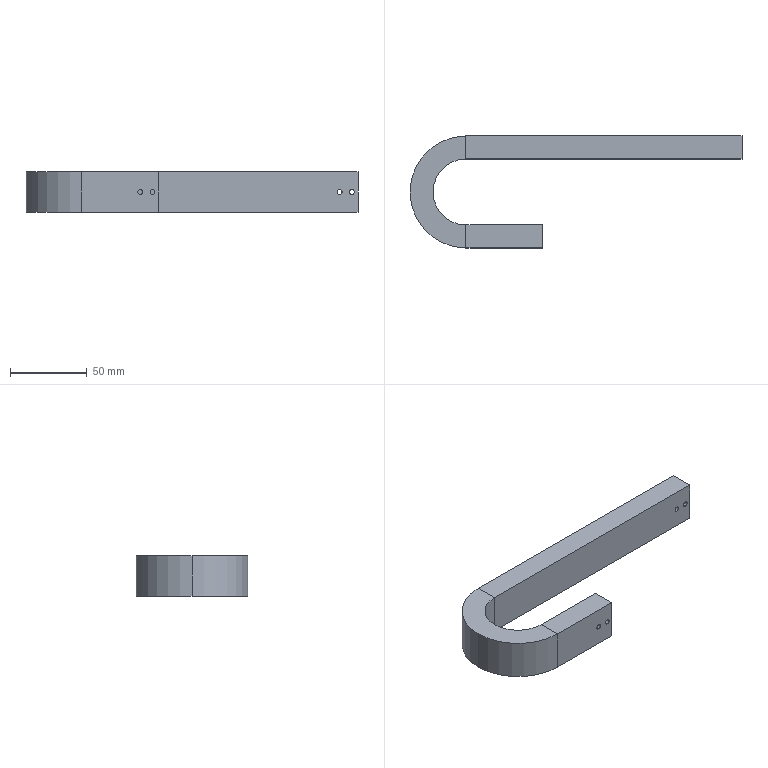Part | NX | features BREP 1 | 1 solid | 50 faces | box 216.5 x 73 x 26.5 mm | volume 63258 mm3 | cylinder 24 | plane 22 | cone 4 | commonest cylinder face diameters 3.2 x16 43 x2 48 x2 68 x2 73 x2
STEP:
#1=CARTESIAN_POINT('',(126.,53.,1.6));
#2=VERTEX_POINT('',#1);
#3=CARTESIAN_POINT('',(126.,50.5,1.6));
#4=VERTEX_POINT('',#3);
#5=CARTESIAN_POINT('',(126.,50.5,1.6));
#6=DIRECTION('',(0.,-1.,0.));
#7=VECTOR('',#6,1000.);
#8=LINE('',#5,#7);
#9=EDGE_CURVE('',#2,#4,#8,.T.);
#10=ORIENTED_EDGE('',*,*,#9,.F.);
#11=CARTESIAN_POINT('',(126.,53.,-1.6));
#12=VERTEX_POINT('',#11);
#13=CARTESIAN_POINT('',(126.,53.,0.));
#14=DIRECTION('',(0.,-1.,0.));
#15=DIRECTION('',(0.,0.,-1.));
#16=AXIS2_PLACEMENT_3D('',#13,#14,#15);
#17=CIRCLE('',#16,1.6);
#18=EDGE_CURVE('',#12,#2,#17,.T.);
#19=ORIENTED_EDGE('',*,*,#18,.F.);
#20=CARTESIAN_POINT('',(126.,50.5,-1.6));
#21=VERTEX_POINT('',#20);
#22=CARTESIAN_POINT('',(126.,50.5,-1.6));
#23=DIRECTION('',(0.,-1.,0.));
#24=VECTOR('',#23,1000.);
#25=LINE('',#22,#24);
#26=EDGE_CURVE('',#12,#21,#25,.T.);
#27=ORIENTED_EDGE('',*,*,#26,.T.);
#28=CARTESIAN_POINT('',(126.,50.5,0.));
#29=DIRECTION('',(0.,-1.,0.));
#30=DIRECTION('',(0.,0.,-1.));
#31=AXIS2_PLACEMENT_3D('',#28,#29,#30);
#32=CIRCLE('',#31,1.6);
#33=EDGE_CURVE('',#21,#4,#32,.T.);
#34=ORIENTED_EDGE('',*,*,#33,.T.);
#35=EDGE_LOOP('',(#10,#19,#27,#34));
#36=FACE_BOUND('',#35,.T.);
#37=CARTESIAN_POINT('',(126.,50.5,0.));
#38=DIRECTION('',(0.,-1.,0.));
#39=DIRECTION('',(0.,0.,-1.));
#40=AXIS2_PLACEMENT_3D('',#37,#38,#39);
#41=CYLINDRICAL_SURFACE('',#40,1.6);
#42=ADVANCED_FACE('',(#36),#41,.F.);
#43=CARTESIAN_POINT('',(126.,65.499,1.6));
#44=VERTEX_POINT('',#43);
#45=CARTESIAN_POINT('',(126.,63.,1.6));
#46=VERTEX_POINT('',#45);
#47=CARTESIAN_POINT('',(126.,50.5,1.6));
#48=DIRECTION('',(0.,-1.,0.));
#49=VECTOR('',#48,1000.);
#50=LINE('',#47,#49);
#51=EDGE_CURVE('',#44,#46,#50,.T.);
#52=ORIENTED_EDGE('',*,*,#51,.F.);
#53=CARTESIAN_POINT('',(126.,65.499,-1.6));
#54=VERTEX_POINT('',#53);
#55=CARTESIAN_POINT('',(126.,65.499,0.));
#56=DIRECTION('',(0.,-1.,0.));
#57=DIRECTION('',(0.,0.,-1.));
#58=AXIS2_PLACEMENT_3D('',#55,#56,#57);
#59=CIRCLE('',#58,1.6);
#60=EDGE_CURVE('',#54,#44,#59,.T.);
#61=ORIENTED_EDGE('',*,*,#60,.F.);
#62=CARTESIAN_POINT('',(126.,63.,-1.6));
#63=VERTEX_POINT('',#62);
#64=CARTESIAN_POINT('',(126.,50.5,-1.6));
#65=DIRECTION('',(0.,-1.,0.));
#66=VECTOR('',#65,1000.);
#67=LINE('',#64,#66);
#68=EDGE_CURVE('',#54,#63,#67,.T.);
#69=ORIENTED_EDGE('',*,*,#68,.T.);
#70=CARTESIAN_POINT('',(126.,63.,0.));
#71=DIRECTION('',(0.,1.,0.));
#72=DIRECTION('',(0.,0.,1.));
#73=AXIS2_PLACEMENT_3D('',#70,#71,#72);
#74=CIRCLE('',#73,1.6);
#75=EDGE_CURVE('',#46,#63,#74,.T.);
#76=ORIENTED_EDGE('',*,*,#75,.F.);
#77=EDGE_LOOP('',(#52,#61,#69,#76));
#78=FACE_BOUND('',#77,.T.);
#79=CARTESIAN_POINT('',(126.,50.5,0.));
#80=DIRECTION('',(0.,-1.,0.));
#81=DIRECTION('',(0.,0.,-1.));
#82=AXIS2_PLACEMENT_3D('',#79,#80,#81);
#83=CYLINDRICAL_SURFACE('',#82,1.6);
#84=ADVANCED_FACE('',(#78),#83,.F.);
#85=CARTESIAN_POINT('',(126.,65.5,1.598));
#86=VERTEX_POINT('',#85);
#87=CARTESIAN_POINT('',(126.,65.499,1.6));
#88=DIRECTION('',(0.,-0.515,0.8572));
#89=VECTOR('',#88,1000.);
#90=LINE('',#87,#89);
#91=EDGE_CURVE('',#86,#44,#90,.T.);
#92=ORIENTED_EDGE('',*,*,#91,.F.);
#93=CARTESIAN_POINT('',(126.,65.5,-1.598));
#94=VERTEX_POINT('',#93);
#95=CARTESIAN_POINT('',(126.,65.5,0.));
#96=DIRECTION('',(0.,-1.,0.));
#97=DIRECTION('',(0.,0.,-1.));
#98=AXIS2_PLACEMENT_3D('',#95,#96,#97);
#99=CIRCLE('',#98,1.598);
#100=EDGE_CURVE('',#94,#86,#99,.T.);
#101=ORIENTED_EDGE('',*,*,#100,.F.);
#102=CARTESIAN_POINT('',(126.,65.499,-1.6));
#103=DIRECTION('',(0.,-0.515,-0.8572));
#104=VECTOR('',#103,1000.);
#105=LINE('',#102,#104);
#106=EDGE_CURVE('',#94,#54,#105,.T.);
#107=ORIENTED_EDGE('',*,*,#106,.T.);
#108=ORIENTED_EDGE('',*,*,#60,.T.);
#109=EDGE_LOOP('',(#92,#101,#107,#108));
#110=FACE_BOUND('',#109,.T.);
#111=CARTESIAN_POINT('',(126.,65.499,0.));
#112=DIRECTION('',(0.,-1.,0.));
#113=DIRECTION('',(0.,0.,-1.));
#114=AXIS2_PLACEMENT_3D('',#111,#112,#113);
#115=CONICAL_SURFACE('',#114,1.6,1.03);
#116=ADVANCED_FACE('',(#110),#115,.F.);
#117=CARTESIAN_POINT('',(118.,65.499,1.6));
#118=VERTEX_POINT('',#117);
#119=CARTESIAN_POINT('',(118.,63.,1.6));
#120=VERTEX_POINT('',#119);
#121=CARTESIAN_POINT('',(118.,50.5,1.6));
#122=DIRECTION('',(0.,-1.,0.));
#123=VECTOR('',#122,1000.);
#124=LINE('',#121,#123);
#125=EDGE_CURVE('',#118,#120,#124,.T.);
#126=ORIENTED_EDGE('',*,*,#125,.F.);
#127=CARTESIAN_POINT('',(118.,65.499,-1.6));
#128=VERTEX_POINT('',#127);
#129=CARTESIAN_POINT('',(118.,65.499,0.));
#130=DIRECTION('',(0.,-1.,0.));
#131=DIRECTION('',(0.,0.,-1.));
#132=AXIS2_PLACEMENT_3D('',#129,#130,#131);
#133=CIRCLE('',#132,1.6);
#134=EDGE_CURVE('',#128,#118,#133,.T.);
#135=ORIENTED_EDGE('',*,*,#134,.F.);
#136=CARTESIAN_POINT('',(118.,63.,-1.6));
#137=VERTEX_POINT('',#136);
#138=CARTESIAN_POINT('',(118.,50.5,-1.6));
#139=DIRECTION('',(0.,-1.,0.));
#140=VECTOR('',#139,1000.);
#141=LINE('',#138,#140);
#142=EDGE_CURVE('',#128,#137,#141,.T.);
#143=ORIENTED_EDGE('',*,*,#142,.T.);
#144=CARTESIAN_POINT('',(118.,63.,0.));
#145=DIRECTION('',(0.,1.,0.));
#146=DIRECTION('',(0.,0.,1.));
#147=AXIS2_PLACEMENT_3D('',#144,#145,#146);
#148=CIRCLE('',#147,1.6);
#149=EDGE_CURVE('',#120,#137,#148,.T.);
#150=ORIENTED_EDGE('',*,*,#149,.F.);
#151=EDGE_LOOP('',(#126,#135,#143,#150));
#152=FACE_BOUND('',#151,.T.);
#153=CARTESIAN_POINT('',(118.,50.5,0.));
#154=DIRECTION('',(0.,-1.,0.));
#155=DIRECTION('',(0.,0.,-1.));
#156=AXIS2_PLACEMENT_3D('',#153,#154,#155);
#157=CYLINDRICAL_SURFACE('',#156,1.6);
#158=ADVANCED_FACE('',(#152),#157,.F.);
#159=CARTESIAN_POINT('',(118.,65.5,1.598));
#160=VERTEX_POINT('',#159);
#161=CARTESIAN_POINT('',(118.,65.499,1.6));
#162=DIRECTION('',(0.,-0.515,0.8572));
#163=VECTOR('',#162,1000.);
#164=LINE('',#161,#163);
#165=EDGE_CURVE('',#160,#118,#164,.T.);
#166=ORIENTED_EDGE('',*,*,#165,.F.);
#167=CARTESIAN_POINT('',(118.,65.5,-1.598));
#168=VERTEX_POINT('',#167);
#169=CARTESIAN_POINT('',(118.,65.5,0.));
#170=DIRECTION('',(0.,-1.,0.));
#171=DIRECTION('',(0.,0.,-1.));
#172=AXIS2_PLACEMENT_3D('',#169,#170,#171);
#173=CIRCLE('',#172,1.598);
#174=EDGE_CURVE('',#168,#160,#173,.T.);
#175=ORIENTED_EDGE('',*,*,#174,.F.);
#176=CARTESIAN_POINT('',(118.,65.499,-1.6));
#177=DIRECTION('',(0.,-0.515,-0.8572));
#178=VECTOR('',#177,1000.);
#179=LINE('',#176,#178);
#180=EDGE_CURVE('',#168,#128,#179,.T.);
#181=ORIENTED_EDGE('',*,*,#180,.T.);
#182=ORIENTED_EDGE('',*,*,#134,.T.);
#183=EDGE_LOOP('',(#166,#175,#181,#182));
#184=FACE_BOUND('',#183,.T.);
#185=CARTESIAN_POINT('',(118.,65.499,0.));
#186=DIRECTION('',(0.,-1.,0.));
#187=DIRECTION('',(0.,0.,-1.));
#188=AXIS2_PLACEMENT_3D('',#185,#186,#187);
#189=CONICAL_SURFACE('',#188,1.6,1.03);
#190=ADVANCED_FACE('',(#184),#189,.F.);
#191=CARTESIAN_POINT('',(118.,53.,1.6));
#192=VERTEX_POINT('',#191);
#193=CARTESIAN_POINT('',(118.,50.5,1.6));
#194=VERTEX_POINT('',#193);
#195=CARTESIAN_POINT('',(118.,50.5,1.6));
#196=DIRECTION('',(0.,-1.,0.));
#197=VECTOR('',#196,1000.);
#198=LINE('',#195,#197);
#199=EDGE_CURVE('',#192,#194,#198,.T.);
#200=ORIENTED_EDGE('',*,*,#199,.F.);
#201=CARTESIAN_POINT('',(118.,53.,-1.6));
#202=VERTEX_POINT('',#201);
#203=CARTESIAN_POINT('',(118.,53.,0.));
#204=DIRECTION('',(0.,-1.,0.));
#205=DIRECTION('',(0.,0.,-1.));
#206=AXIS2_PLACEMENT_3D('',#203,#204,#205);
#207=CIRCLE('',#206,1.6);
#208=EDGE_CURVE('',#202,#192,#207,.T.);
#209=ORIENTED_EDGE('',*,*,#208,.F.);
#210=CARTESIAN_POINT('',(118.,50.5,-1.6));
#211=VERTEX_POINT('',#210);
#212=CARTESIAN_POINT('',(118.,50.5,-1.6));
#213=DIRECTION('',(0.,-1.,0.));
#214=VECTOR('',#213,1000.);
#215=LINE('',#212,#214);
#216=EDGE_CURVE('',#202,#211,#215,.T.);
#217=ORIENTED_EDGE('',*,*,#216,.T.);
#218=CARTESIAN_POINT('',(118.,50.5,0.));
#219=DIRECTION('',(0.,-1.,0.));
#220=DIRECTION('',(0.,0.,-1.));
#221=AXIS2_PLACEMENT_3D('',#218,#219,#220);
#222=CIRCLE('',#221,1.6);
#223=EDGE_CURVE('',#211,#194,#222,.T.);
#224=ORIENTED_EDGE('',*,*,#223,.T.);
#225=EDGE_LOOP('',(#200,#209,#217,#224));
#226=FACE_BOUND('',#225,.T.);
#227=CARTESIAN_POINT('',(118.,50.5,0.));
#228=DIRECTION('',(0.,-1.,0.));
#229=DIRECTION('',(0.,0.,-1.));
#230=AXIS2_PLACEMENT_3D('',#227,#228,#229);
#231=CYLINDRICAL_SURFACE('',#230,1.6);
#232=ADVANCED_FACE('',(#226),#231,.F.);
#233=CARTESIAN_POINT('',(-4.,7.5,1.6));
#234=VERTEX_POINT('',#233);
#235=CARTESIAN_POINT('',(-4.,5.,1.6));
#236=VERTEX_POINT('',#235);
#237=CARTESIAN_POINT('',(-4.,-7.5,1.6));
#238=DIRECTION('',(0.,-1.,0.));
#239=VECTOR('',#238,1000.);
#240=LINE('',#237,#239);
#241=EDGE_CURVE('',#234,#236,#240,.T.);
#242=ORIENTED_EDGE('',*,*,#241,.F.);
#243=CARTESIAN_POINT('',(-4.,7.5,-1.6));
#244=VERTEX_POINT('',#243);
#245=CARTESIAN_POINT('',(-4.,7.5,0.));
#246=DIRECTION('',(0.,1.,0.));
#247=DIRECTION('',(1.,0.,0.));
#248=AXIS2_PLACEMENT_3D('',#245,#246,#247);
#249=CIRCLE('',#248,1.6);
#250=EDGE_CURVE('',#234,#244,#249,.T.);
#251=ORIENTED_EDGE('',*,*,#250,.T.);
#252=CARTESIAN_POINT('',(-4.,5.,-1.6));
#253=VERTEX_POINT('',#252);
#254=CARTESIAN_POINT('',(-4.,-7.5,-1.6));
#255=DIRECTION('',(0.,-1.,0.));
#256=VECTOR('',#255,1000.);
#257=LINE('',#254,#256);
#258=EDGE_CURVE('',#244,#253,#257,.T.);
#259=ORIENTED_EDGE('',*,*,#258,.T.);
#260=CARTESIAN_POINT('',(-4.,5.,0.));
#261=DIRECTION('',(0.,1.,0.));
#262=DIRECTION('',(-1.,0.,0.));
#263=AXIS2_PLACEMENT_3D('',#260,#261,#262);
#264=CIRCLE('',#263,1.6);
#265=EDGE_CURVE('',#236,#253,#264,.T.);
#266=ORIENTED_EDGE('',*,*,#265,.F.);
#267=EDGE_LOOP('',(#242,#251,#259,#266));
#268=FACE_BOUND('',#267,.T.);
#269=CARTESIAN_POINT('',(-4.,-7.5,0.));
#270=DIRECTION('',(0.,-1.,0.));
#271=DIRECTION('',(0.,0.,-1.));
#272=AXIS2_PLACEMENT_3D('',#269,#270,#271);
#273=CYLINDRICAL_SURFACE('',#272,1.6);
#274=ADVANCED_FACE('',(#268),#273,.F.);
#275=CARTESIAN_POINT('',(-4.,-5.,1.6));
#276=VERTEX_POINT('',#275);
#277=CARTESIAN_POINT('',(-4.,-7.5,1.6));
#278=VERTEX_POINT('',#277);
#279=CARTESIAN_POINT('',(-4.,-7.5,1.6));
#280=DIRECTION('',(0.,-1.,0.));
#281=VECTOR('',#280,1000.);
#282=LINE('',#279,#281);
#283=EDGE_CURVE('',#276,#278,#282,.T.);
#284=ORIENTED_EDGE('',*,*,#283,.F.);
#285=CARTESIAN_POINT('',(-4.,-5.,-1.6));
#286=VERTEX_POINT('',#285);
#287=CARTESIAN_POINT('',(-4.,-5.,0.));
#288=DIRECTION('',(0.,-1.,0.));
#289=DIRECTION('',(1.,0.,0.));
#290=AXIS2_PLACEMENT_3D('',#287,#288,#289);
#291=CIRCLE('',#290,1.6);
#292=EDGE_CURVE('',#286,#276,#291,.T.);
#293=ORIENTED_EDGE('',*,*,#292,.F.);
#294=CARTESIAN_POINT('',(-4.,-7.5,-1.6));
#295=VERTEX_POINT('',#294);
#296=CARTESIAN_POINT('',(-4.,-7.5,-1.6));
#297=DIRECTION('',(0.,-1.,0.));
#298=VECTOR('',#297,1000.);
#299=LINE('',#296,#298);
#300=EDGE_CURVE('',#286,#295,#299,.T.);
#301=ORIENTED_EDGE('',*,*,#300,.T.);
#302=CARTESIAN_POINT('',(-4.,-7.5,0.));
#303=DIRECTION('',(0.,-1.,0.));
#304=DIRECTION('',(0.,0.,-1.));
#305=AXIS2_PLACEMENT_3D('',#302,#303,#304);
#306=CIRCLE('',#305,1.6);
#307=EDGE_CURVE('',#295,#278,#306,.T.);
#308=ORIENTED_EDGE('',*,*,#307,.T.);
#309=EDGE_LOOP('',(#284,#293,#301,#308));
#310=FACE_BOUND('',#309,.T.);
#311=CARTESIAN_POINT('',(-4.,-7.5,0.));
#312=DIRECTION('',(0.,-1.,0.));
#313=DIRECTION('',(0.,0.,-1.));
#314=AXIS2_PLACEMENT_3D('',#311,#312,#313);
#315=CYLINDRICAL_SURFACE('',#314,1.6);
#316=ADVANCED_FACE('',(#310),#315,.F.);
#317=CARTESIAN_POINT('',(-12.,7.5,1.6));
#318=VERTEX_POINT('',#317);
#319=CARTESIAN_POINT('',(-12.,5.,1.6));
#320=VERTEX_POINT('',#319);
#321=CARTESIAN_POINT('',(-12.,-7.5,1.6));
#322=DIRECTION('',(0.,-1.,0.));
#323=VECTOR('',#322,1000.);
#324=LINE('',#321,#323);
#325=EDGE_CURVE('',#318,#320,#324,.T.);
#326=ORIENTED_EDGE('',*,*,#325,.F.);
#327=CARTESIAN_POINT('',(-12.,7.5,-1.6));
#328=VERTEX_POINT('',#327);
#329=CARTESIAN_POINT('',(-12.,7.5,0.));
#330=DIRECTION('',(0.,1.,0.));
#331=DIRECTION('',(1.,0.,0.));
#332=AXIS2_PLACEMENT_3D('',#329,#330,#331);
#333=CIRCLE('',#332,1.6);
#334=EDGE_CURVE('',#318,#328,#333,.T.);
#335=ORIENTED_EDGE('',*,*,#334,.T.);
#336=CARTESIAN_POINT('',(-12.,5.,-1.6));
#337=VERTEX_POINT('',#336);
#338=CARTESIAN_POINT('',(-12.,-7.5,-1.6));
#339=DIRECTION('',(0.,-1.,0.));
#340=VECTOR('',#339,1000.);
#341=LINE('',#338,#340);
#342=EDGE_CURVE('',#328,#337,#341,.T.);
#343=ORIENTED_EDGE('',*,*,#342,.T.);
#344=CARTESIAN_POINT('',(-12.,5.,0.));
#345=DIRECTION('',(0.,1.,0.));
#346=DIRECTION('',(-1.,0.,0.));
#347=AXIS2_PLACEMENT_3D('',#344,#345,#346);
#348=CIRCLE('',#347,1.6);
#349=EDGE_CURVE('',#320,#337,#348,.T.);
#350=ORIENTED_EDGE('',*,*,#349,.F.);
#351=EDGE_LOOP('',(#326,#335,#343,#350));
#352=FACE_BOUND('',#351,.T.);
#353=CARTESIAN_POINT('',(-12.,-7.5,0.));
#354=DIRECTION('',(0.,-1.,0.));
#355=DIRECTION('',(0.,0.,-1.));
#356=AXIS2_PLACEMENT_3D('',#353,#354,#355);
#357=CYLINDRICAL_SURFACE('',#356,1.6);
#358=ADVANCED_FACE('',(#352),#357,.F.);
#359=CARTESIAN_POINT('',(-12.,-5.,1.6));
#360=VERTEX_POINT('',#359);
#361=CARTESIAN_POINT('',(-12.,-7.5,1.6));
#362=VERTEX_POINT('',#361);
#363=CARTESIAN_POINT('',(-12.,-7.5,1.6));
#364=DIRECTION('',(0.,-1.,0.));
#365=VECTOR('',#364,1000.);
#366=LINE('',#363,#365);
#367=EDGE_CURVE('',#360,#362,#366,.T.);
#368=ORIENTED_EDGE('',*,*,#367,.F.);
#369=CARTESIAN_POINT('',(-12.,-5.,-1.6));
#370=VERTEX_POINT('',#369);
#371=CARTESIAN_POINT('',(-12.,-5.,0.));
#372=DIRECTION('',(0.,-1.,0.));
#373=DIRECTION('',(1.,0.,0.));
#374=AXIS2_PLACEMENT_3D('',#371,#372,#373);
#375=CIRCLE('',#374,1.6);
#376=EDGE_CURVE('',#370,#360,#375,.T.);
#377=ORIENTED_EDGE('',*,*,#376,.F.);
#378=CARTESIAN_POINT('',(-12.,-7.5,-1.6));
#379=VERTEX_POINT('',#378);
#380=CARTESIAN_POINT('',(-12.,-7.5,-1.6));
#381=DIRECTION('',(0.,-1.,0.));
#382=VECTOR('',#381,1000.);
#383=LINE('',#380,#382);
#384=EDGE_CURVE('',#370,#379,#383,.T.);
#385=ORIENTED_EDGE('',*,*,#384,.T.);
#386=CARTESIAN_POINT('',(-12.,-7.5,0.));
#387=DIRECTION('',(0.,-1.,0.));
#388=DIRECTION('',(0.,0.,-1.));
#389=AXIS2_PLACEMENT_3D('',#386,#387,#388);
#390=CIRCLE('',#389,1.6);
#391=EDGE_CURVE('',#379,#362,#390,.T.);
#392=ORIENTED_EDGE('',*,*,#391,.T.);
#393=EDGE_LOOP('',(#368,#377,#385,#392));
#394=FACE_BOUND('',#393,.T.);
#395=CARTESIAN_POINT('',(-12.,-7.5,0.));
#396=DIRECTION('',(0.,-1.,0.));
#397=DIRECTION('',(0.,0.,-1.));
#398=AXIS2_PLACEMENT_3D('',#395,#396,#397);
#399=CYLINDRICAL_SURFACE('',#398,1.6);
#400=ADVANCED_FACE('',(#394),#399,.F.);
#401=CARTESIAN_POINT('',(0.,7.5,-13.25));
#402=VERTEX_POINT('',#401);
#403=CARTESIAN_POINT('',(-50.,7.5,-13.25));
#404=VERTEX_POINT('',#403);
#405=CARTESIAN_POINT('',(0.,7.5,-13.25));
#406=DIRECTION('',(-1.,0.,0.));
#407=VECTOR('',#406,1000.);
#408=LINE('',#405,#407);
#409=EDGE_CURVE('',#402,#404,#408,.T.);
#410=ORIENTED_EDGE('',*,*,#409,.F.);
#411=CARTESIAN_POINT('',(0.,-7.5,-13.25));
#412=VERTEX_POINT('',#411);
#413=CARTESIAN_POINT('',(0.,-7.5,-13.25));
#414=DIRECTION('',(0.,1.,0.));
#415=VECTOR('',#414,1000.);
#416=LINE('',#413,#415);
#417=EDGE_CURVE('',#412,#402,#416,.T.);
#418=ORIENTED_EDGE('',*,*,#417,.F.);
#419=CARTESIAN_POINT('',(-50.,-7.5,-13.25));
#420=VERTEX_POINT('',#419);
#421=CARTESIAN_POINT('',(0.,-7.5,-13.25));
#422=DIRECTION('',(-1.,0.,0.));
#423=VECTOR('',#422,1000.);
#424=LINE('',#421,#423);
#425=EDGE_CURVE('',#412,#420,#424,.T.);
#426=ORIENTED_EDGE('',*,*,#425,.T.);
#427=CARTESIAN_POINT('',(-50.,-7.5,-13.25));
#428=DIRECTION('',(0.,1.,0.));
#429=VECTOR('',#428,1000.);
#430=LINE('',#427,#429);
#431=EDGE_CURVE('',#420,#404,#430,.T.);
#432=ORIENTED_EDGE('',*,*,#431,.T.);
#433=EDGE_LOOP('',(#410,#418,#426,#432));
#434=FACE_BOUND('',#433,.T.);
#435=CARTESIAN_POINT('',(0.,-7.5,-13.25));
#436=DIRECTION('',(0.,0.,1.));
#437=DIRECTION('',(1.,0.,0.));
#438=AXIS2_PLACEMENT_3D('',#435,#436,#437);
#439=PLANE('',#438);
#440=ADVANCED_FACE('',(#434),#439,.F.);
#441=CARTESIAN_POINT('',(0.,-7.5,13.25));
#442=VERTEX_POINT('',#441);
#443=CARTESIAN_POINT('',(-50.,-7.5,13.25));
#444=VERTEX_POINT('',#443);
#445=CARTESIAN_POINT('',(0.,-7.5,13.25));
#446=DIRECTION('',(-1.,0.,0.));
#447=VECTOR('',#446,1000.);
#448=LINE('',#445,#447);
#449=EDGE_CURVE('',#442,#444,#448,.T.);
#450=ORIENTED_EDGE('',*,*,#449,.F.);
#451=CARTESIAN_POINT('',(0.,7.5,13.25));
#452=VERTEX_POINT('',#451);
#453=CARTESIAN_POINT('',(0.,-7.5,13.25));
#454=DIRECTION('',(0.,-1.,0.));
#455=VECTOR('',#454,1000.);
#456=LINE('',#453,#455);
#457=EDGE_CURVE('',#452,#442,#456,.T.);
#458=ORIENTED_EDGE('',*,*,#457,.F.);
#459=CARTESIAN_POINT('',(-50.,7.5,13.25));
#460=VERTEX_POINT('',#459);
#461=CARTESIAN_POINT('',(0.,7.5,13.25));
#462=DIRECTION('',(-1.,0.,0.));
#463=VECTOR('',#462,1000.);
#464=LINE('',#461,#463);
#465=EDGE_CURVE('',#452,#460,#464,.T.);
#466=ORIENTED_EDGE('',*,*,#465,.T.);
#467=CARTESIAN_POINT('',(-50.,-7.5,13.25));
#468=DIRECTION('',(0.,-1.,0.));
#469=VECTOR('',#468,1000.);
#470=LINE('',#467,#469);
#471=EDGE_CURVE('',#460,#444,#470,.T.);
#472=ORIENTED_EDGE('',*,*,#471,.T.);
#473=EDGE_LOOP('',(#450,#458,#466,#472));
#474=FACE_BOUND('',#473,.T.);
#475=CARTESIAN_POINT('',(0.,-7.5,13.25));
#476=DIRECTION('',(0.,0.,-1.));
#477=DIRECTION('',(-1.,0.,0.));
#478=AXIS2_PLACEMENT_3D('',#475,#476,#477);
#479=PLANE('',#478);
#480=ADVANCED_FACE('',(#474),#479,.F.);
#481=CARTESIAN_POINT('',(-50.,-7.5,13.25));
#482=DIRECTION('',(0.,0.,-1.));
#483=VECTOR('',#482,1000.);
#484=LINE('',#481,#483);
#485=EDGE_CURVE('',#444,#420,#484,.T.);
#486=ORIENTED_EDGE('',*,*,#485,.T.);
#487=ORIENTED_EDGE('',*,*,#425,.F.);
#488=CARTESIAN_POINT('',(0.,-7.5,13.25));
#489=DIRECTION('',(0.,0.,-1.));
#490=VECTOR('',#489,1000.);
#491=LINE('',#488,#490);
#492=EDGE_CURVE('',#442,#412,#491,.T.);
#493=ORIENTED_EDGE('',*,*,#492,.F.);
#494=ORIENTED_EDGE('',*,*,#449,.T.);
#495=EDGE_LOOP('',(#486,#487,#493,#494));
#496=FACE_BOUND('',#495,.T.);
#497=ORIENTED_EDGE('',*,*,#391,.F.);
#498=CARTESIAN_POINT('',(-12.,-7.5,0.));
#499=DIRECTION('',(0.,-1.,0.));
#500=DIRECTION('',(0.,0.,-1.));
#501=AXIS2_PLACEMENT_3D('',#498,#499,#500);
#502=CIRCLE('',#501,1.6);
#503=EDGE_CURVE('',#362,#379,#502,.T.);
#504=ORIENTED_EDGE('',*,*,#503,.F.);
#505=EDGE_LOOP('',(#497,#504));
#506=FACE_BOUND('',#505,.T.);
#507=ORIENTED_EDGE('',*,*,#307,.F.);
#508=CARTESIAN_POINT('',(-4.,-7.5,0.));
#509=DIRECTION('',(0.,-1.,0.));
#510=DIRECTION('',(0.,0.,-1.));
#511=AXIS2_PLACEMENT_3D('',#508,#509,#510);
#512=CIRCLE('',#511,1.6);
#513=EDGE_CURVE('',#278,#295,#512,.T.);
#514=ORIENTED_EDGE('',*,*,#513,.F.);
#515=EDGE_LOOP('',(#507,#514));
#516=FACE_BOUND('',#515,.T.);
#517=CARTESIAN_POINT('',(0.,-7.5,13.25));
#518=DIRECTION('',(0.,1.,0.));
#519=DIRECTION('',(-1.,0.,0.));
#520=AXIS2_PLACEMENT_3D('',#517,#518,#519);
#521=PLANE('',#520);
#522=ADVANCED_FACE('',(#496,#506,#516),#521,.F.);
#523=CARTESIAN_POINT('',(-71.5,29.,-13.25));
#524=VERTEX_POINT('',#523);
#525=CARTESIAN_POINT('',(-50.,29.,-13.25));
#526=DIRECTION('',(0.,0.,-1.));
#527=DIRECTION('',(0.,-1.,0.));
#528=AXIS2_PLACEMENT_3D('',#525,#526,#527);
#529=CIRCLE('',#528,21.5);
#530=EDGE_CURVE('',#404,#524,#529,.T.);
#531=ORIENTED_EDGE('',*,*,#530,.F.);
#532=ORIENTED_EDGE('',*,*,#431,.F.);
#533=CARTESIAN_POINT('',(-86.5,29.,-13.25));
#534=VERTEX_POINT('',#533);
#535=CARTESIAN_POINT('',(-50.,29.,-13.25));
#536=DIRECTION('',(0.,0.,-1.));
#537=DIRECTION('',(0.,-1.,0.));
#538=AXIS2_PLACEMENT_3D('',#535,#536,#537);
#539=CIRCLE('',#538,36.5);
#540=EDGE_CURVE('',#420,#534,#539,.T.);
#541=ORIENTED_EDGE('',*,*,#540,.T.);
#542=CARTESIAN_POINT('',(-50.,65.5,-13.25));
#543=VERTEX_POINT('',#542);
#544=CARTESIAN_POINT('',(-50.,29.,-13.25));
#545=DIRECTION('',(0.,0.,-1.));
#546=DIRECTION('',(0.,-1.,0.));
#547=AXIS2_PLACEMENT_3D('',#544,#545,#546);
#548=CIRCLE('',#547,36.5);
#549=EDGE_CURVE('',#534,#543,#548,.T.);
#550=ORIENTED_EDGE('',*,*,#549,.T.);
#551=CARTESIAN_POINT('',(-50.,50.5,-13.25));
#552=VERTEX_POINT('',#551);
#553=CARTESIAN_POINT('',(-50.,65.5,-13.25));
#554=DIRECTION('',(0.,-1.,0.));
#555=VECTOR('',#554,1000.);
#556=LINE('',#553,#555);
#557=EDGE_CURVE('',#543,#552,#556,.T.);
#558=ORIENTED_EDGE('',*,*,#557,.T.);
#559=CARTESIAN_POINT('',(-50.,29.,-13.25));
#560=DIRECTION('',(0.,0.,-1.));
#561=DIRECTION('',(0.,-1.,0.));
#562=AXIS2_PLACEMENT_3D('',#559,#560,#561);
#563=CIRCLE('',#562,21.5);
#564=EDGE_CURVE('',#524,#552,#563,.T.);
#565=ORIENTED_EDGE('',*,*,#564,.F.);
#566=EDGE_LOOP('',(#531,#532,#541,#550,#558,#565));
#567=FACE_BOUND('',#566,.T.);
#568=CARTESIAN_POINT('',(-50.,-7.5,-13.25));
#569=DIRECTION('',(0.,0.,1.));
#570=DIRECTION('',(1.,0.,0.));
#571=AXIS2_PLACEMENT_3D('',#568,#569,#570);
#572=PLANE('',#571);
#573=ADVANCED_FACE('',(#567),#572,.F.);
#574=CARTESIAN_POINT('',(-71.5,29.,13.25));
#575=VERTEX_POINT('',#574);
#576=CARTESIAN_POINT('',(-71.5,29.,0.));
#577=DIRECTION('',(0.,0.,-1.));
#578=VECTOR('',#577,1000.);
#579=LINE('',#576,#578);
#580=EDGE_CURVE('',#575,#524,#579,.T.);
#581=ORIENTED_EDGE('',*,*,#580,.F.);
#582=CARTESIAN_POINT('',(-50.,29.,13.25));
#583=DIRECTION('',(0.,0.,-1.));
#584=DIRECTION('',(0.,-1.,0.));
#585=AXIS2_PLACEMENT_3D('',#582,#583,#584);
#586=CIRCLE('',#585,21.5);
#587=EDGE_CURVE('',#460,#575,#586,.T.);
#588=ORIENTED_EDGE('',*,*,#587,.F.);
#589=CARTESIAN_POINT('',(-50.,7.5,13.25));
#590=DIRECTION('',(0.,0.,1.));
#591=VECTOR('',#590,1000.);
#592=LINE('',#589,#591);
#593=EDGE_CURVE('',#404,#460,#592,.T.);
#594=ORIENTED_EDGE('',*,*,#593,.F.);
#595=ORIENTED_EDGE('',*,*,#530,.T.);
#596=EDGE_LOOP('',(#581,#588,#594,#595));
#597=FACE_BOUND('',#596,.T.);
#598=CARTESIAN_POINT('',(-50.,29.,0.));
#599=DIRECTION('',(0.,0.,-1.));
#600=DIRECTION('',(-1.,0.,0.));
#601=AXIS2_PLACEMENT_3D('',#598,#599,#600);
#602=CYLINDRICAL_SURFACE('',#601,21.5);
#603=ADVANCED_FACE('',(#597),#602,.F.);
#604=CARTESIAN_POINT('',(-86.5,29.,13.25));
#605=VERTEX_POINT('',#604);
#606=CARTESIAN_POINT('',(-50.,29.,13.25));
#607=DIRECTION('',(0.,0.,-1.));
#608=DIRECTION('',(0.,-1.,0.));
#609=AXIS2_PLACEMENT_3D('',#606,#607,#608);
#610=CIRCLE('',#609,36.5);
#611=EDGE_CURVE('',#444,#605,#610,.T.);
#612=ORIENTED_EDGE('',*,*,#611,.F.);
#613=ORIENTED_EDGE('',*,*,#471,.F.);
#614=ORIENTED_EDGE('',*,*,#587,.T.);
#615=CARTESIAN_POINT('',(-50.,50.5,13.25));
#616=VERTEX_POINT('',#615);
#617=CARTESIAN_POINT('',(-50.,29.,13.25));
#618=DIRECTION('',(0.,0.,-1.));
#619=DIRECTION('',(0.,-1.,0.));
#620=AXIS2_PLACEMENT_3D('',#617,#618,#619);
#621=CIRCLE('',#620,21.5);
#622=EDGE_CURVE('',#575,#616,#621,.T.);
#623=ORIENTED_EDGE('',*,*,#622,.T.);
#624=CARTESIAN_POINT('',(-50.,65.5,13.25));
#625=VERTEX_POINT('',#624);
#626=CARTESIAN_POINT('',(-50.,65.5,13.25));
#627=DIRECTION('',(0.,1.,0.));
#628=VECTOR('',#627,1000.);
#629=LINE('',#626,#628);
#630=EDGE_CURVE('',#616,#625,#629,.T.);
#631=ORIENTED_EDGE('',*,*,#630,.T.);
#632=CARTESIAN_POINT('',(-50.,29.,13.25));
#633=DIRECTION('',(0.,0.,-1.));
#634=DIRECTION('',(0.,-1.,0.));
#635=AXIS2_PLACEMENT_3D('',#632,#633,#634);
#636=CIRCLE('',#635,36.5);
#637=EDGE_CURVE('',#605,#625,#636,.T.);
#638=ORIENTED_EDGE('',*,*,#637,.F.);
#639=EDGE_LOOP('',(#612,#613,#614,#623,#631,#638));
#640=FACE_BOUND('',#639,.T.);
#641=CARTESIAN_POINT('',(-50.,-7.5,13.25));
#642=DIRECTION('',(0.,0.,-1.));
#643=DIRECTION('',(-1.,0.,0.));
#644=AXIS2_PLACEMENT_3D('',#641,#642,#643);
#645=PLANE('',#644);
#646=ADVANCED_FACE('',(#640),#645,.F.);
#647=CARTESIAN_POINT('',(-86.5,29.,0.));
#648=DIRECTION('',(0.,0.,-1.));
#649=VECTOR('',#648,1000.);
#650=LINE('',#647,#649);
#651=EDGE_CURVE('',#605,#534,#650,.T.);
#652=ORIENTED_EDGE('',*,*,#651,.F.);
#653=ORIENTED_EDGE('',*,*,#637,.T.);
#654=CARTESIAN_POINT('',(-50.,65.5,13.25));
#655=DIRECTION('',(0.,0.,-1.));
#656=VECTOR('',#655,1000.);
#657=LINE('',#654,#656);
#658=EDGE_CURVE('',#625,#543,#657,.T.);
#659=ORIENTED_EDGE('',*,*,#658,.T.);
#660=ORIENTED_EDGE('',*,*,#549,.F.);
#661=EDGE_LOOP('',(#652,#653,#659,#660));
#662=FACE_BOUND('',#661,.T.);
#663=CARTESIAN_POINT('',(-50.,29.,0.));
#664=DIRECTION('',(0.,0.,-1.));
#665=DIRECTION('',(-1.,0.,0.));
#666=AXIS2_PLACEMENT_3D('',#663,#664,#665);
#667=CYLINDRICAL_SURFACE('',#666,36.5);
#668=ADVANCED_FACE('',(#662),#667,.T.);
#669=CARTESIAN_POINT('',(130.,50.5,-13.25));
#670=VERTEX_POINT('',#669);
#671=CARTESIAN_POINT('',(-50.,50.5,-13.25));
#672=DIRECTION('',(1.,0.,0.));
#673=VECTOR('',#672,1000.);
#674=LINE('',#671,#673);
#675=EDGE_CURVE('',#552,#670,#674,.T.);
#676=ORIENTED_EDGE('',*,*,#675,.F.);
#677=ORIENTED_EDGE('',*,*,#557,.F.);
#678=CARTESIAN_POINT('',(130.,65.5,-13.25));
#679=VERTEX_POINT('',#678);
#680=CARTESIAN_POINT('',(-50.,65.5,-13.25));
#681=DIRECTION('',(1.,0.,0.));
#682=VECTOR('',#681,1000.);
#683=LINE('',#680,#682);
#684=EDGE_CURVE('',#543,#679,#683,.T.);
#685=ORIENTED_EDGE('',*,*,#684,.T.);
#686=CARTESIAN_POINT('',(130.,65.5,-13.25));
#687=DIRECTION('',(0.,-1.,0.));
#688=VECTOR('',#687,1000.);
#689=LINE('',#686,#688);
#690=EDGE_CURVE('',#679,#670,#689,.T.);
#691=ORIENTED_EDGE('',*,*,#690,.T.);
#692=EDGE_LOOP('',(#676,#677,#685,#691));
#693=FACE_BOUND('',#692,.T.);
#694=CARTESIAN_POINT('',(-50.,65.5,-13.25));
#695=DIRECTION('',(0.,0.,1.));
#696=DIRECTION('',(1.,0.,0.));
#697=AXIS2_PLACEMENT_3D('',#694,#695,#696);
#698=PLANE('',#697);
#699=ADVANCED_FACE('',(#693),#698,.F.);
#700=CARTESIAN_POINT('',(130.,50.5,13.25));
#701=VERTEX_POINT('',#700);
#702=CARTESIAN_POINT('',(-50.,50.5,13.25));
#703=DIRECTION('',(1.,0.,0.));
#704=VECTOR('',#703,1000.);
#705=LINE('',#702,#704);
#706=EDGE_CURVE('',#616,#701,#705,.T.);
#707=ORIENTED_EDGE('',*,*,#706,.F.);
#708=CARTESIAN_POINT('',(-50.,50.5,13.25));
#709=DIRECTION('',(0.,0.,1.));
#710=VECTOR('',#709,1000.);
#711=LINE('',#708,#710);
#712=EDGE_CURVE('',#552,#616,#711,.T.);
#713=ORIENTED_EDGE('',*,*,#712,.F.);
#714=ORIENTED_EDGE('',*,*,#675,.T.);
#715=CARTESIAN_POINT('',(130.,50.5,13.25));
#716=DIRECTION('',(0.,0.,1.));
#717=VECTOR('',#716,1000.);
#718=LINE('',#715,#717);
#719=EDGE_CURVE('',#670,#701,#718,.T.);
#720=ORIENTED_EDGE('',*,*,#719,.T.);
#721=EDGE_LOOP('',(#707,#713,#714,#720));
#722=FACE_BOUND('',#721,.T.);
#723=ORIENTED_EDGE('',*,*,#223,.F.);
#724=CARTESIAN_POINT('',(118.,50.5,0.));
#725=DIRECTION('',(0.,-1.,0.));
#726=DIRECTION('',(0.,0.,-1.));
#727=AXIS2_PLACEMENT_3D('',#724,#725,#726);
#728=CIRCLE('',#727,1.6);
#729=EDGE_CURVE('',#194,#211,#728,.T.);
#730=ORIENTED_EDGE('',*,*,#729,.F.);
#731=EDGE_LOOP('',(#723,#730));
#732=FACE_BOUND('',#731,.T.);
#733=ORIENTED_EDGE('',*,*,#33,.F.);
#734=CARTESIAN_POINT('',(126.,50.5,0.));
#735=DIRECTION('',(0.,-1.,0.));
#736=DIRECTION('',(0.,0.,-1.));
#737=AXIS2_PLACEMENT_3D('',#734,#735,#736);
#738=CIRCLE('',#737,1.6);
#739=EDGE_CURVE('',#4,#21,#738,.T.);
#740=ORIENTED_EDGE('',*,*,#739,.F.);
#741=EDGE_LOOP('',(#733,#740));
#742=FACE_BOUND('',#741,.T.);
#743=CARTESIAN_POINT('',(-50.,50.5,13.25));
#744=DIRECTION('',(0.,1.,0.));
#745=DIRECTION('',(0.,0.,1.));
#746=AXIS2_PLACEMENT_3D('',#743,#744,#745);
#747=PLANE('',#746);
#748=ADVANCED_FACE('',(#722,#732,#742),#747,.F.);
#749=CARTESIAN_POINT('',(130.,65.5,13.25));
#750=VERTEX_POINT('',#749);
#751=CARTESIAN_POINT('',(-50.,65.5,13.25));
#752=DIRECTION('',(1.,0.,0.));
#753=VECTOR('',#752,1000.);
#754=LINE('',#751,#753);
#755=EDGE_CURVE('',#625,#750,#754,.T.);
#756=ORIENTED_EDGE('',*,*,#755,.F.);
#757=ORIENTED_EDGE('',*,*,#630,.F.);
#758=ORIENTED_EDGE('',*,*,#706,.T.);
#759=CARTESIAN_POINT('',(130.,65.5,13.25));
#760=DIRECTION('',(0.,1.,0.));
#761=VECTOR('',#760,1000.);
#762=LINE('',#759,#761);
#763=EDGE_CURVE('',#701,#750,#762,.T.);
#764=ORIENTED_EDGE('',*,*,#763,.T.);
#765=EDGE_LOOP('',(#756,#757,#758,#764));
#766=FACE_BOUND('',#765,.T.);
#767=CARTESIAN_POINT('',(-50.,65.5,13.25));
#768=DIRECTION('',(0.,0.,-1.));
#769=DIRECTION('',(-1.,0.,0.));
#770=AXIS2_PLACEMENT_3D('',#767,#768,#769);
#771=PLANE('',#770);
#772=ADVANCED_FACE('',(#766),#771,.F.);
#773=CARTESIAN_POINT('',(130.,65.5,13.25));
#774=DIRECTION('',(0.,0.,-1.));
#775=VECTOR('',#774,1000.);
#776=LINE('',#773,#775);
#777=EDGE_CURVE('',#750,#679,#776,.T.);
#778=ORIENTED_EDGE('',*,*,#777,.T.);
#779=ORIENTED_EDGE('',*,*,#684,.F.);
#780=ORIENTED_EDGE('',*,*,#658,.F.);
#781=ORIENTED_EDGE('',*,*,#755,.T.);
#782=EDGE_LOOP('',(#778,#779,#780,#781));
#783=FACE_BOUND('',#782,.T.);
#784=ORIENTED_EDGE('',*,*,#174,.T.);
#785=CARTESIAN_POINT('',(118.,65.5,0.));
#786=DIRECTION('',(0.,-1.,0.));
#787=DIRECTION('',(0.,0.,-1.));
#788=AXIS2_PLACEMENT_3D('',#785,#786,#787);
#789=CIRCLE('',#788,1.598);
#790=EDGE_CURVE('',#160,#168,#789,.T.);
#791=ORIENTED_EDGE('',*,*,#790,.T.);
#792=EDGE_LOOP('',(#784,#791));
#793=FACE_BOUND('',#792,.T.);
#794=ORIENTED_EDGE('',*,*,#100,.T.);
#795=CARTESIAN_POINT('',(126.,65.5,0.));
#796=DIRECTION('',(0.,-1.,0.));
#797=DIRECTION('',(0.,0.,-1.));
#798=AXIS2_PLACEMENT_3D('',#795,#796,#797);
#799=CIRCLE('',#798,1.598);
#800=EDGE_CURVE('',#86,#94,#799,.T.);
#801=ORIENTED_EDGE('',*,*,#800,.T.);
#802=EDGE_LOOP('',(#794,#801));
#803=FACE_BOUND('',#802,.T.);
#804=CARTESIAN_POINT('',(-50.,65.5,13.25));
#805=DIRECTION('',(0.,-1.,0.));
#806=DIRECTION('',(0.,0.,-1.));
#807=AXIS2_PLACEMENT_3D('',#804,#805,#806);
#808=PLANE('',#807);
#809=ADVANCED_FACE('',(#783,#793,#803),#808,.F.);
#810=CARTESIAN_POINT('',(0.,5.,-10.));
#811=VERTEX_POINT('',#810);
#812=CARTESIAN_POINT('',(0.,-5.,-10.));
#813=VERTEX_POINT('',#812);
#814=CARTESIAN_POINT('',(0.,-5.,-10.));
#815=DIRECTION('',(0.,-1.,0.));
#816=VECTOR('',#815,1000.);
#817=LINE('',#814,#816);
#818=EDGE_CURVE('',#811,#813,#817,.T.);
#819=ORIENTED_EDGE('',*,*,#818,.T.);
#820=CARTESIAN_POINT('',(0.,-5.,10.));
#821=VERTEX_POINT('',#820);
#822=CARTESIAN_POINT('',(0.,-5.,10.));
#823=DIRECTION('',(0.,0.,1.));
#824=VECTOR('',#823,1000.);
#825=LINE('',#822,#824);
#826=EDGE_CURVE('',#813,#821,#825,.T.);
#827=ORIENTED_EDGE('',*,*,#826,.T.);
#828=CARTESIAN_POINT('',(0.,5.,10.));
#829=VERTEX_POINT('',#828);
#830=CARTESIAN_POINT('',(0.,-5.,10.));
#831=DIRECTION('',(0.,1.,0.));
#832=VECTOR('',#831,1000.);
#833=LINE('',#830,#832);
#834=EDGE_CURVE('',#821,#829,#833,.T.);
#835=ORIENTED_EDGE('',*,*,#834,.T.);
#836=CARTESIAN_POINT('',(0.,5.,10.));
#837=DIRECTION('',(0.,0.,-1.));
#838=VECTOR('',#837,1000.);
#839=LINE('',#836,#838);
#840=EDGE_CURVE('',#829,#811,#839,.T.);
#841=ORIENTED_EDGE('',*,*,#840,.T.);
#842=EDGE_LOOP('',(#819,#827,#835,#841));
#843=FACE_BOUND('',#842,.T.);
#844=ORIENTED_EDGE('',*,*,#417,.T.);
#845=CARTESIAN_POINT('',(0.,7.5,13.25));
#846=DIRECTION('',(0.,0.,1.));
#847=VECTOR('',#846,1000.);
#848=LINE('',#845,#847);
#849=EDGE_CURVE('',#402,#452,#848,.T.);
#850=ORIENTED_EDGE('',*,*,#849,.T.);
#851=ORIENTED_EDGE('',*,*,#457,.T.);
#852=ORIENTED_EDGE('',*,*,#492,.T.);
#853=EDGE_LOOP('',(#844,#850,#851,#852));
#854=FACE_BOUND('',#853,.T.);
#855=CARTESIAN_POINT('',(0.,0.,0.));
#856=DIRECTION('',(-1.,0.,0.));
#857=DIRECTION('',(0.,0.,1.));
#858=AXIS2_PLACEMENT_3D('',#855,#856,#857);
#859=PLANE('',#858);
#860=ADVANCED_FACE('',(#843,#854),#859,.F.);
#861=CARTESIAN_POINT('',(130.,53.,-10.));
#862=VERTEX_POINT('',#861);
#863=CARTESIAN_POINT('',(130.,63.,-10.));
#864=VERTEX_POINT('',#863);
#865=CARTESIAN_POINT('',(130.,63.,-10.));
#866=DIRECTION('',(0.,1.,0.));
#867=VECTOR('',#866,1000.);
#868=LINE('',#865,#867);
#869=EDGE_CURVE('',#862,#864,#868,.T.);
#870=ORIENTED_EDGE('',*,*,#869,.F.);
#871=CARTESIAN_POINT('',(130.,53.,10.));
#872=VERTEX_POINT('',#871);
#873=CARTESIAN_POINT('',(130.,53.,10.));
#874=DIRECTION('',(0.,0.,-1.));
#875=VECTOR('',#874,1000.);
#876=LINE('',#873,#875);
#877=EDGE_CURVE('',#872,#862,#876,.T.);
#878=ORIENTED_EDGE('',*,*,#877,.F.);
#879=CARTESIAN_POINT('',(130.,63.,10.));
#880=VERTEX_POINT('',#879);
#881=CARTESIAN_POINT('',(130.,63.,10.));
#882=DIRECTION('',(0.,-1.,0.));
#883=VECTOR('',#882,1000.);
#884=LINE('',#881,#883);
#885=EDGE_CURVE('',#880,#872,#884,.T.);
#886=ORIENTED_EDGE('',*,*,#885,.F.);
#887=CARTESIAN_POINT('',(130.,63.,10.));
#888=DIRECTION('',(0.,0.,1.));
#889=VECTOR('',#888,1000.);
#890=LINE('',#887,#889);
#891=EDGE_CURVE('',#864,#880,#890,.T.);
#892=ORIENTED_EDGE('',*,*,#891,.F.);
#893=EDGE_LOOP('',(#870,#878,#886,#892));
#894=FACE_BOUND('',#893,.T.);
#895=ORIENTED_EDGE('',*,*,#690,.F.);
#896=ORIENTED_EDGE('',*,*,#777,.F.);
#897=ORIENTED_EDGE('',*,*,#763,.F.);
#898=ORIENTED_EDGE('',*,*,#719,.F.);
#899=EDGE_LOOP('',(#895,#896,#897,#898));
#900=FACE_BOUND('',#899,.T.);
#901=CARTESIAN_POINT('',(130.,58.,0.));
#902=DIRECTION('',(1.,0.,0.));
#903=DIRECTION('',(0.,0.,1.));
#904=AXIS2_PLACEMENT_3D('',#901,#902,#903);
#905=PLANE('',#904);
#906=ADVANCED_FACE('',(#894,#900),#905,.T.);
#907=CARTESIAN_POINT('',(-50.,-5.,10.));
#908=VERTEX_POINT('',#907);
#909=CARTESIAN_POINT('',(0.,-5.,10.));
#910=DIRECTION('',(-1.,0.,0.));
#911=VECTOR('',#910,1000.);
#912=LINE('',#909,#911);
#913=EDGE_CURVE('',#821,#908,#912,.T.);
#914=ORIENTED_EDGE('',*,*,#913,.F.);
#915=ORIENTED_EDGE('',*,*,#826,.F.);
#916=CARTESIAN_POINT('',(-50.,-5.,-10.));
#917=VERTEX_POINT('',#916);
#918=CARTESIAN_POINT('',(0.,-5.,-10.));
#919=DIRECTION('',(-1.,0.,0.));
#920=VECTOR('',#919,1000.);
#921=LINE('',#918,#920);
#922=EDGE_CURVE('',#813,#917,#921,.T.);
#923=ORIENTED_EDGE('',*,*,#922,.T.);
#924=CARTESIAN_POINT('',(-50.,-5.,10.));
#925=DIRECTION('',(0.,0.,1.));
#926=VECTOR('',#925,1000.);
#927=LINE('',#924,#926);
#928=EDGE_CURVE('',#917,#908,#927,.T.);
#929=ORIENTED_EDGE('',*,*,#928,.T.);
#930=EDGE_LOOP('',(#914,#915,#923,#929));
#931=FACE_BOUND('',#930,.T.);
#932=ORIENTED_EDGE('',*,*,#376,.T.);
#933=CARTESIAN_POINT('',(-12.,-5.,0.));
#934=DIRECTION('',(0.,-1.,0.));
#935=DIRECTION('',(1.,0.,0.));
#936=AXIS2_PLACEMENT_3D('',#933,#934,#935);
#937=CIRCLE('',#936,1.6);
#938=EDGE_CURVE('',#360,#370,#937,.T.);
#939=ORIENTED_EDGE('',*,*,#938,.T.);
#940=EDGE_LOOP('',(#932,#939));
#941=FACE_BOUND('',#940,.T.);
#942=ORIENTED_EDGE('',*,*,#292,.T.);
#943=CARTESIAN_POINT('',(-4.,-5.,0.));
#944=DIRECTION('',(0.,-1.,0.));
#945=DIRECTION('',(1.,0.,0.));
#946=AXIS2_PLACEMENT_3D('',#943,#944,#945);
#947=CIRCLE('',#946,1.6);
#948=EDGE_CURVE('',#276,#286,#947,.T.);
#949=ORIENTED_EDGE('',*,*,#948,.T.);
#950=EDGE_LOOP('',(#942,#949));
#951=FACE_BOUND('',#950,.T.);
#952=CARTESIAN_POINT('',(0.,-5.,10.));
#953=DIRECTION('',(0.,-1.,0.));
#954=DIRECTION('',(1.,0.,0.));
#955=AXIS2_PLACEMENT_3D('',#952,#953,#954);
#956=PLANE('',#955);
#957=ADVANCED_FACE('',(#931,#941,#951),#956,.F.);
#958=CARTESIAN_POINT('',(-50.,5.,10.));
#959=VERTEX_POINT('',#958);
#960=CARTESIAN_POINT('',(0.,5.,10.));
#961=DIRECTION('',(-1.,0.,0.));
#962=VECTOR('',#961,1000.);
#963=LINE('',#960,#962);
#964=EDGE_CURVE('',#829,#959,#963,.T.);
#965=ORIENTED_EDGE('',*,*,#964,.F.);
#966=ORIENTED_EDGE('',*,*,#834,.F.);
#967=ORIENTED_EDGE('',*,*,#913,.T.);
#968=CARTESIAN_POINT('',(-50.,-5.,10.));
#969=DIRECTION('',(0.,1.,0.));
#970=VECTOR('',#969,1000.);
#971=LINE('',#968,#970);
#972=EDGE_CURVE('',#908,#959,#971,.T.);
#973=ORIENTED_EDGE('',*,*,#972,.T.);
#974=EDGE_LOOP('',(#965,#966,#967,#973));
#975=FACE_BOUND('',#974,.T.);
#976=CARTESIAN_POINT('',(0.,-5.,10.));
#977=DIRECTION('',(0.,0.,1.));
#978=DIRECTION('',(1.,0.,0.));
#979=AXIS2_PLACEMENT_3D('',#976,#977,#978);
#980=PLANE('',#979);
#981=ADVANCED_FACE('',(#975),#980,.F.);
#982=CARTESIAN_POINT('',(-50.,5.,-10.));
#983=VERTEX_POINT('',#982);
#984=CARTESIAN_POINT('',(0.,5.,-10.));
#985=DIRECTION('',(-1.,0.,0.));
#986=VECTOR('',#985,1000.);
#987=LINE('',#984,#986);
#988=EDGE_CURVE('',#811,#983,#987,.T.);
#989=ORIENTED_EDGE('',*,*,#988,.F.);
#990=ORIENTED_EDGE('',*,*,#840,.F.);
#991=ORIENTED_EDGE('',*,*,#964,.T.);
#992=CARTESIAN_POINT('',(-50.,5.,10.));
#993=DIRECTION('',(0.,0.,-1.));
#994=VECTOR('',#993,1000.);
#995=LINE('',#992,#994);
#996=EDGE_CURVE('',#959,#983,#995,.T.);
#997=ORIENTED_EDGE('',*,*,#996,.T.);
#998=EDGE_LOOP('',(#989,#990,#991,#997));
#999=FACE_BOUND('',#998,.T.);
#1000=CARTESIAN_POINT('',(-12.,5.,0.));
#1001=DIRECTION('',(0.,1.,0.));
#1002=DIRECTION('',(-1.,0.,0.));
#1003=AXIS2_PLACEMENT_3D('',#1000,#1001,#1002);
#1004=CIRCLE('',#1003,1.6);
#1005=EDGE_CURVE('',#337,#320,#1004,.T.);
#1006=ORIENTED_EDGE('',*,*,#1005,.T.);
#1007=ORIENTED_EDGE('',*,*,#349,.T.);
#1008=EDGE_LOOP('',(#1006,#1007));
#1009=FACE_BOUND('',#1008,.T.);
#1010=CARTESIAN_POINT('',(-4.,5.,0.));
#1011=DIRECTION('',(0.,1.,0.));
#1012=DIRECTION('',(-1.,0.,0.));
#1013=AXIS2_PLACEMENT_3D('',#1010,#1011,#1012);
#1014=CIRCLE('',#1013,1.6);
#1015=EDGE_CURVE('',#253,#236,#1014,.T.);
#1016=ORIENTED_EDGE('',*,*,#1015,.T.);
#1017=ORIENTED_EDGE('',*,*,#265,.T.);
#1018=EDGE_LOOP('',(#1016,#1017));
#1019=FACE_BOUND('',#1018,.T.);
#1020=CARTESIAN_POINT('',(0.,5.,10.));
#1021=DIRECTION('',(0.,1.,0.));
#1022=DIRECTION('',(-1.,0.,0.));
#1023=AXIS2_PLACEMENT_3D('',#1020,#1021,#1022);
#1024=PLANE('',#1023);
#1025=ADVANCED_FACE('',(#999,#1009,#1019),#1024,.F.);
#1026=CARTESIAN_POINT('',(-50.,-5.,-10.));
#1027=DIRECTION('',(0.,-1.,0.));
#1028=VECTOR('',#1027,1000.);
#1029=LINE('',#1026,#1028);
#1030=EDGE_CURVE('',#983,#917,#1029,.T.);
#1031=ORIENTED_EDGE('',*,*,#1030,.T.);
#1032=ORIENTED_EDGE('',*,*,#922,.F.);
#1033=ORIENTED_EDGE('',*,*,#818,.F.);
#1034=ORIENTED_EDGE('',*,*,#988,.T.);
#1035=EDGE_LOOP('',(#1031,#1032,#1033,#1034));
#1036=FACE_BOUND('',#1035,.T.);
#1037=CARTESIAN_POINT('',(0.,-5.,-10.));
#1038=DIRECTION('',(0.,0.,-1.));
#1039=DIRECTION('',(-1.,0.,0.));
#1040=AXIS2_PLACEMENT_3D('',#1037,#1038,#1039);
#1041=PLANE('',#1040);
#1042=ADVANCED_FACE('',(#1036),#1041,.F.);
#1043=CARTESIAN_POINT('',(-84.,29.,10.));
#1044=VERTEX_POINT('',#1043);
#1045=CARTESIAN_POINT('',(-84.,29.,-10.));
#1046=VERTEX_POINT('',#1045);
#1047=CARTESIAN_POINT('',(-84.,29.,0.));
#1048=DIRECTION('',(0.,0.,-1.));
#1049=VECTOR('',#1048,1000.);
#1050=LINE('',#1047,#1049);
#1051=EDGE_CURVE('',#1044,#1046,#1050,.T.);
#1052=ORIENTED_EDGE('',*,*,#1051,.F.);
#1053=CARTESIAN_POINT('',(-50.,29.,10.));
#1054=DIRECTION('',(0.,0.,-1.));
#1055=DIRECTION('',(0.,-1.,0.));
#1056=AXIS2_PLACEMENT_3D('',#1053,#1054,#1055);
#1057=CIRCLE('',#1056,34.);
#1058=EDGE_CURVE('',#908,#1044,#1057,.T.);
#1059=ORIENTED_EDGE('',*,*,#1058,.F.);
#1060=ORIENTED_EDGE('',*,*,#928,.F.);
#1061=CARTESIAN_POINT('',(-50.,29.,-10.));
#1062=DIRECTION('',(0.,0.,-1.));
#1063=DIRECTION('',(0.,-1.,0.));
#1064=AXIS2_PLACEMENT_3D('',#1061,#1062,#1063);
#1065=CIRCLE('',#1064,34.);
#1066=EDGE_CURVE('',#917,#1046,#1065,.T.);
#1067=ORIENTED_EDGE('',*,*,#1066,.T.);
#1068=EDGE_LOOP('',(#1052,#1059,#1060,#1067));
#1069=FACE_BOUND('',#1068,.T.);
#1070=CARTESIAN_POINT('',(-50.,29.,0.));
#1071=DIRECTION('',(0.,0.,-1.));
#1072=DIRECTION('',(-1.,0.,0.));
#1073=AXIS2_PLACEMENT_3D('',#1070,#1071,#1072);
#1074=CYLINDRICAL_SURFACE('',#1073,34.);
#1075=ADVANCED_FACE('',(#1069),#1074,.F.);
#1076=CARTESIAN_POINT('',(-74.,29.,10.));
#1077=VERTEX_POINT('',#1076);
#1078=CARTESIAN_POINT('',(-50.,29.,10.));
#1079=DIRECTION('',(0.,0.,-1.));
#1080=DIRECTION('',(0.,-1.,0.));
#1081=AXIS2_PLACEMENT_3D('',#1078,#1079,#1080);
#1082=CIRCLE('',#1081,24.);
#1083=EDGE_CURVE('',#959,#1077,#1082,.T.);
#1084=ORIENTED_EDGE('',*,*,#1083,.F.);
#1085=ORIENTED_EDGE('',*,*,#972,.F.);
#1086=ORIENTED_EDGE('',*,*,#1058,.T.);
#1087=CARTESIAN_POINT('',(-50.,63.,10.));
#1088=VERTEX_POINT('',#1087);
#1089=CARTESIAN_POINT('',(-50.,29.,10.));
#1090=DIRECTION('',(0.,0.,-1.));
#1091=DIRECTION('',(0.,-1.,0.));
#1092=AXIS2_PLACEMENT_3D('',#1089,#1090,#1091);
#1093=CIRCLE('',#1092,34.);
#1094=EDGE_CURVE('',#1044,#1088,#1093,.T.);
#1095=ORIENTED_EDGE('',*,*,#1094,.T.);
#1096=CARTESIAN_POINT('',(-50.,53.,10.));
#1097=VERTEX_POINT('',#1096);
#1098=CARTESIAN_POINT('',(-50.,63.,10.));
#1099=DIRECTION('',(0.,-1.,0.));
#1100=VECTOR('',#1099,1000.);
#1101=LINE('',#1098,#1100);
#1102=EDGE_CURVE('',#1088,#1097,#1101,.T.);
#1103=ORIENTED_EDGE('',*,*,#1102,.T.);
#1104=CARTESIAN_POINT('',(-50.,29.,10.));
#1105=DIRECTION('',(0.,0.,-1.));
#1106=DIRECTION('',(0.,-1.,0.));
#1107=AXIS2_PLACEMENT_3D('',#1104,#1105,#1106);
#1108=CIRCLE('',#1107,24.);
#1109=EDGE_CURVE('',#1077,#1097,#1108,.T.);
#1110=ORIENTED_EDGE('',*,*,#1109,.F.);
#1111=EDGE_LOOP('',(#1084,#1085,#1086,#1095,#1103,#1110));
#1112=FACE_BOUND('',#1111,.T.);
#1113=CARTESIAN_POINT('',(-50.,-5.,10.));
#1114=DIRECTION('',(0.,0.,1.));
#1115=DIRECTION('',(1.,0.,0.));
#1116=AXIS2_PLACEMENT_3D('',#1113,#1114,#1115);
#1117=PLANE('',#1116);
#1118=ADVANCED_FACE('',(#1112),#1117,.F.);
#1119=CARTESIAN_POINT('',(-74.,29.,-10.));
#1120=VERTEX_POINT('',#1119);
#1121=CARTESIAN_POINT('',(-74.,29.,0.));
#1122=DIRECTION('',(0.,0.,-1.));
#1123=VECTOR('',#1122,1000.);
#1124=LINE('',#1121,#1123);
#1125=EDGE_CURVE('',#1077,#1120,#1124,.T.);
#1126=ORIENTED_EDGE('',*,*,#1125,.F.);
#1127=ORIENTED_EDGE('',*,*,#1109,.T.);
#1128=CARTESIAN_POINT('',(-50.,53.,-10.));
#1129=VERTEX_POINT('',#1128);
#1130=CARTESIAN_POINT('',(-50.,53.,10.));
#1131=DIRECTION('',(0.,0.,-1.));
#1132=VECTOR('',#1131,1000.);
#1133=LINE('',#1130,#1132);
#1134=EDGE_CURVE('',#1097,#1129,#1133,.T.);
#1135=ORIENTED_EDGE('',*,*,#1134,.T.);
#1136=CARTESIAN_POINT('',(-50.,29.,-10.));
#1137=DIRECTION('',(0.,0.,-1.));
#1138=DIRECTION('',(0.,-1.,0.));
#1139=AXIS2_PLACEMENT_3D('',#1136,#1137,#1138);
#1140=CIRCLE('',#1139,24.);
#1141=EDGE_CURVE('',#1120,#1129,#1140,.T.);
#1142=ORIENTED_EDGE('',*,*,#1141,.F.);
#1143=EDGE_LOOP('',(#1126,#1127,#1135,#1142));
#1144=FACE_BOUND('',#1143,.T.);
#1145=CARTESIAN_POINT('',(-50.,29.,0.));
#1146=DIRECTION('',(0.,0.,-1.));
#1147=DIRECTION('',(-1.,0.,0.));
#1148=AXIS2_PLACEMENT_3D('',#1145,#1146,#1147);
#1149=CYLINDRICAL_SURFACE('',#1148,24.);
#1150=ADVANCED_FACE('',(#1144),#1149,.T.);
#1151=CARTESIAN_POINT('',(-50.,63.,-10.));
#1152=VERTEX_POINT('',#1151);
#1153=CARTESIAN_POINT('',(-50.,63.,-10.));
#1154=DIRECTION('',(0.,1.,0.));
#1155=VECTOR('',#1154,1000.);
#1156=LINE('',#1153,#1155);
#1157=EDGE_CURVE('',#1129,#1152,#1156,.T.);
#1158=ORIENTED_EDGE('',*,*,#1157,.T.);
#1159=CARTESIAN_POINT('',(-50.,29.,-10.));
#1160=DIRECTION('',(0.,0.,-1.));
#1161=DIRECTION('',(0.,-1.,0.));
#1162=AXIS2_PLACEMENT_3D('',#1159,#1160,#1161);
#1163=CIRCLE('',#1162,34.);
#1164=EDGE_CURVE('',#1046,#1152,#1163,.T.);
#1165=ORIENTED_EDGE('',*,*,#1164,.F.);
#1166=ORIENTED_EDGE('',*,*,#1066,.F.);
#1167=ORIENTED_EDGE('',*,*,#1030,.F.);
#1168=CARTESIAN_POINT('',(-50.,29.,-10.));
#1169=DIRECTION('',(0.,0.,-1.));
#1170=DIRECTION('',(0.,-1.,0.));
#1171=AXIS2_PLACEMENT_3D('',#1168,#1169,#1170);
#1172=CIRCLE('',#1171,24.);
#1173=EDGE_CURVE('',#983,#1120,#1172,.T.);
#1174=ORIENTED_EDGE('',*,*,#1173,.T.);
#1175=ORIENTED_EDGE('',*,*,#1141,.T.);
#1176=EDGE_LOOP('',(#1158,#1165,#1166,#1167,#1174,#1175));
#1177=FACE_BOUND('',#1176,.T.);
#1178=CARTESIAN_POINT('',(-50.,-5.,-10.));
#1179=DIRECTION('',(0.,0.,-1.));
#1180=DIRECTION('',(-1.,0.,0.));
#1181=AXIS2_PLACEMENT_3D('',#1178,#1179,#1180);
#1182=PLANE('',#1181);
#1183=ADVANCED_FACE('',(#1177),#1182,.F.);
#1184=CARTESIAN_POINT('',(-50.,63.,10.));
#1185=DIRECTION('',(1.,0.,0.));
#1186=VECTOR('',#1185,1000.);
#1187=LINE('',#1184,#1186);
#1188=EDGE_CURVE('',#1088,#880,#1187,.T.);
#1189=ORIENTED_EDGE('',*,*,#1188,.F.);
#1190=CARTESIAN_POINT('',(-50.,63.,10.));
#1191=DIRECTION('',(0.,0.,1.));
#1192=VECTOR('',#1191,1000.);
#1193=LINE('',#1190,#1192);
#1194=EDGE_CURVE('',#1152,#1088,#1193,.T.);
#1195=ORIENTED_EDGE('',*,*,#1194,.F.);
#1196=CARTESIAN_POINT('',(-50.,63.,-10.));
#1197=DIRECTION('',(1.,0.,0.));
#1198=VECTOR('',#1197,1000.);
#1199=LINE('',#1196,#1198);
#1200=EDGE_CURVE('',#1152,#864,#1199,.T.);
#1201=ORIENTED_EDGE('',*,*,#1200,.T.);
#1202=ORIENTED_EDGE('',*,*,#891,.T.);
#1203=EDGE_LOOP('',(#1189,#1195,#1201,#1202));
#1204=FACE_BOUND('',#1203,.T.);
#1205=CARTESIAN_POINT('',(118.,63.,0.));
#1206=DIRECTION('',(0.,1.,0.));
#1207=DIRECTION('',(0.,0.,1.));
#1208=AXIS2_PLACEMENT_3D('',#1205,#1206,#1207);
#1209=CIRCLE('',#1208,1.6);
#1210=EDGE_CURVE('',#137,#120,#1209,.T.);
#1211=ORIENTED_EDGE('',*,*,#1210,.T.);
#1212=ORIENTED_EDGE('',*,*,#149,.T.);
#1213=EDGE_LOOP('',(#1211,#1212));
#1214=FACE_BOUND('',#1213,.T.);
#1215=CARTESIAN_POINT('',(126.,63.,0.));
#1216=DIRECTION('',(0.,1.,0.));
#1217=DIRECTION('',(0.,0.,1.));
#1218=AXIS2_PLACEMENT_3D('',#1215,#1216,#1217);
#1219=CIRCLE('',#1218,1.6);
#1220=EDGE_CURVE('',#63,#46,#1219,.T.);
#1221=ORIENTED_EDGE('',*,*,#1220,.T.);
#1222=ORIENTED_EDGE('',*,*,#75,.T.);
#1223=EDGE_LOOP('',(#1221,#1222));
#1224=FACE_BOUND('',#1223,.T.);
#1225=CARTESIAN_POINT('',(-50.,63.,10.));
#1226=DIRECTION('',(0.,1.,0.));
#1227=DIRECTION('',(0.,0.,1.));
#1228=AXIS2_PLACEMENT_3D('',#1225,#1226,#1227);
#1229=PLANE('',#1228);
#1230=ADVANCED_FACE('',(#1204,#1214,#1224),#1229,.F.);
#1231=CARTESIAN_POINT('',(-50.,53.,10.));
#1232=DIRECTION('',(1.,0.,0.));
#1233=VECTOR('',#1232,1000.);
#1234=LINE('',#1231,#1233);
#1235=EDGE_CURVE('',#1097,#872,#1234,.T.);
#1236=ORIENTED_EDGE('',*,*,#1235,.F.);
#1237=ORIENTED_EDGE('',*,*,#1102,.F.);
#1238=ORIENTED_EDGE('',*,*,#1188,.T.);
#1239=ORIENTED_EDGE('',*,*,#885,.T.);
#1240=EDGE_LOOP('',(#1236,#1237,#1238,#1239));
#1241=FACE_BOUND('',#1240,.T.);
#1242=CARTESIAN_POINT('',(-50.,63.,10.));
#1243=DIRECTION('',(0.,0.,1.));
#1244=DIRECTION('',(1.,0.,0.));
#1245=AXIS2_PLACEMENT_3D('',#1242,#1243,#1244);
#1246=PLANE('',#1245);
#1247=ADVANCED_FACE('',(#1241),#1246,.F.);
#1248=CARTESIAN_POINT('',(-50.,53.,-10.));
#1249=DIRECTION('',(1.,0.,0.));
#1250=VECTOR('',#1249,1000.);
#1251=LINE('',#1248,#1250);
#1252=EDGE_CURVE('',#1129,#862,#1251,.T.);
#1253=ORIENTED_EDGE('',*,*,#1252,.F.);
#1254=ORIENTED_EDGE('',*,*,#1134,.F.);
#1255=ORIENTED_EDGE('',*,*,#1235,.T.);
#1256=ORIENTED_EDGE('',*,*,#877,.T.);
#1257=EDGE_LOOP('',(#1253,#1254,#1255,#1256));
#1258=FACE_BOUND('',#1257,.T.);
#1259=ORIENTED_EDGE('',*,*,#208,.T.);
#1260=CARTESIAN_POINT('',(118.,53.,0.));
#1261=DIRECTION('',(0.,-1.,0.));
#1262=DIRECTION('',(0.,0.,-1.));
#1263=AXIS2_PLACEMENT_3D('',#1260,#1261,#1262);
#1264=CIRCLE('',#1263,1.6);
#1265=EDGE_CURVE('',#192,#202,#1264,.T.);
#1266=ORIENTED_EDGE('',*,*,#1265,.T.);
#1267=EDGE_LOOP('',(#1259,#1266));
#1268=FACE_BOUND('',#1267,.T.);
#1269=ORIENTED_EDGE('',*,*,#18,.T.);
#1270=CARTESIAN_POINT('',(126.,53.,0.));
#1271=DIRECTION('',(0.,-1.,0.));
#1272=DIRECTION('',(0.,0.,-1.));
#1273=AXIS2_PLACEMENT_3D('',#1270,#1271,#1272);
#1274=CIRCLE('',#1273,1.6);
#1275=EDGE_CURVE('',#2,#12,#1274,.T.);
#1276=ORIENTED_EDGE('',*,*,#1275,.T.);
#1277=EDGE_LOOP('',(#1269,#1276));
#1278=FACE_BOUND('',#1277,.T.);
#1279=CARTESIAN_POINT('',(-50.,53.,10.));
#1280=DIRECTION('',(0.,-1.,0.));
#1281=DIRECTION('',(0.,0.,-1.));
#1282=AXIS2_PLACEMENT_3D('',#1279,#1280,#1281);
#1283=PLANE('',#1282);
#1284=ADVANCED_FACE('',(#1258,#1268,#1278),#1283,.F.);
#1285=ORIENTED_EDGE('',*,*,#869,.T.);
#1286=ORIENTED_EDGE('',*,*,#1200,.F.);
#1287=ORIENTED_EDGE('',*,*,#1157,.F.);
#1288=ORIENTED_EDGE('',*,*,#1252,.T.);
#1289=EDGE_LOOP('',(#1285,#1286,#1287,#1288));
#1290=FACE_BOUND('',#1289,.T.);
#1291=CARTESIAN_POINT('',(-50.,63.,-10.));
#1292=DIRECTION('',(0.,0.,-1.));
#1293=DIRECTION('',(-1.,0.,0.));
#1294=AXIS2_PLACEMENT_3D('',#1291,#1292,#1293);
#1295=PLANE('',#1294);
#1296=ADVANCED_FACE('',(#1290),#1295,.F.);
#1297=CARTESIAN_POINT('',(-4.,7.5,0.));
#1298=DIRECTION('',(0.,1.,0.));
#1299=DIRECTION('',(1.,0.,0.));
#1300=AXIS2_PLACEMENT_3D('',#1297,#1298,#1299);
#1301=CIRCLE('',#1300,1.6);
#1302=EDGE_CURVE('',#244,#234,#1301,.T.);
#1303=ORIENTED_EDGE('',*,*,#1302,.F.);
#1304=ORIENTED_EDGE('',*,*,#250,.F.);
#1305=EDGE_LOOP('',(#1303,#1304));
#1306=FACE_BOUND('',#1305,.T.);
#1307=ORIENTED_EDGE('',*,*,#465,.F.);
#1308=ORIENTED_EDGE('',*,*,#849,.F.);
#1309=ORIENTED_EDGE('',*,*,#409,.T.);
#1310=ORIENTED_EDGE('',*,*,#593,.T.);
#1311=EDGE_LOOP('',(#1307,#1308,#1309,#1310));
#1312=FACE_BOUND('',#1311,.T.);
#1313=CARTESIAN_POINT('',(-12.,7.5,0.));
#1314=DIRECTION('',(0.,1.,0.));
#1315=DIRECTION('',(1.,0.,0.));
#1316=AXIS2_PLACEMENT_3D('',#1313,#1314,#1315);
#1317=CIRCLE('',#1316,1.6);
#1318=EDGE_CURVE('',#328,#318,#1317,.T.);
#1319=ORIENTED_EDGE('',*,*,#1318,.F.);
#1320=ORIENTED_EDGE('',*,*,#334,.F.);
#1321=EDGE_LOOP('',(#1319,#1320));
#1322=FACE_BOUND('',#1321,.T.);
#1323=CARTESIAN_POINT('',(0.,7.5,13.25));
#1324=DIRECTION('',(0.,-1.,0.));
#1325=DIRECTION('',(1.,0.,0.));
#1326=AXIS2_PLACEMENT_3D('',#1323,#1324,#1325);
#1327=PLANE('',#1326);
#1328=ADVANCED_FACE('',(#1306,#1312,#1322),#1327,.F.);
#1329=ORIENTED_EDGE('',*,*,#622,.F.);
#1330=ORIENTED_EDGE('',*,*,#580,.T.);
#1331=ORIENTED_EDGE('',*,*,#564,.T.);
#1332=ORIENTED_EDGE('',*,*,#712,.T.);
#1333=EDGE_LOOP('',(#1329,#1330,#1331,#1332));
#1334=FACE_BOUND('',#1333,.T.);
#1335=CARTESIAN_POINT('',(-50.,29.,0.));
#1336=DIRECTION('',(0.,0.,-1.));
#1337=DIRECTION('',(-1.,0.,0.));
#1338=AXIS2_PLACEMENT_3D('',#1335,#1336,#1337);
#1339=CYLINDRICAL_SURFACE('',#1338,21.5);
#1340=ADVANCED_FACE('',(#1334),#1339,.F.);
#1341=ORIENTED_EDGE('',*,*,#611,.T.);
#1342=ORIENTED_EDGE('',*,*,#651,.T.);
#1343=ORIENTED_EDGE('',*,*,#540,.F.);
#1344=ORIENTED_EDGE('',*,*,#485,.F.);
#1345=EDGE_LOOP('',(#1341,#1342,#1343,#1344));
#1346=FACE_BOUND('',#1345,.T.);
#1347=CARTESIAN_POINT('',(-50.,29.,0.));
#1348=DIRECTION('',(0.,0.,-1.));
#1349=DIRECTION('',(-1.,0.,0.));
#1350=AXIS2_PLACEMENT_3D('',#1347,#1348,#1349);
#1351=CYLINDRICAL_SURFACE('',#1350,36.5);
#1352=ADVANCED_FACE('',(#1346),#1351,.T.);
#1353=ORIENTED_EDGE('',*,*,#1094,.F.);
#1354=ORIENTED_EDGE('',*,*,#1051,.T.);
#1355=ORIENTED_EDGE('',*,*,#1164,.T.);
#1356=ORIENTED_EDGE('',*,*,#1194,.T.);
#1357=EDGE_LOOP('',(#1353,#1354,#1355,#1356));
#1358=FACE_BOUND('',#1357,.T.);
#1359=CARTESIAN_POINT('',(-50.,29.,0.));
#1360=DIRECTION('',(0.,0.,-1.));
#1361=DIRECTION('',(-1.,0.,0.));
#1362=AXIS2_PLACEMENT_3D('',#1359,#1360,#1361);
#1363=CYLINDRICAL_SURFACE('',#1362,34.);
#1364=ADVANCED_FACE('',(#1358),#1363,.F.);
#1365=ORIENTED_EDGE('',*,*,#1083,.T.);
#1366=ORIENTED_EDGE('',*,*,#1125,.T.);
#1367=ORIENTED_EDGE('',*,*,#1173,.F.);
#1368=ORIENTED_EDGE('',*,*,#996,.F.);
#1369=EDGE_LOOP('',(#1365,#1366,#1367,#1368));
#1370=FACE_BOUND('',#1369,.T.);
#1371=CARTESIAN_POINT('',(-50.,29.,0.));
#1372=DIRECTION('',(0.,0.,-1.));
#1373=DIRECTION('',(-1.,0.,0.));
#1374=AXIS2_PLACEMENT_3D('',#1371,#1372,#1373);
#1375=CYLINDRICAL_SURFACE('',#1374,24.);
#1376=ADVANCED_FACE('',(#1370),#1375,.T.);
#1377=ORIENTED_EDGE('',*,*,#938,.F.);
#1378=ORIENTED_EDGE('',*,*,#367,.T.);
#1379=ORIENTED_EDGE('',*,*,#503,.T.);
#1380=ORIENTED_EDGE('',*,*,#384,.F.);
#1381=EDGE_LOOP('',(#1377,#1378,#1379,#1380));
#1382=FACE_BOUND('',#1381,.T.);
#1383=CARTESIAN_POINT('',(-12.,-7.5,0.));
#1384=DIRECTION('',(0.,-1.,0.));
#1385=DIRECTION('',(0.,0.,-1.));
#1386=AXIS2_PLACEMENT_3D('',#1383,#1384,#1385);
#1387=CYLINDRICAL_SURFACE('',#1386,1.6);
#1388=ADVANCED_FACE('',(#1382),#1387,.F.);
#1389=ORIENTED_EDGE('',*,*,#1318,.T.);
#1390=ORIENTED_EDGE('',*,*,#325,.T.);
#1391=ORIENTED_EDGE('',*,*,#1005,.F.);
#1392=ORIENTED_EDGE('',*,*,#342,.F.);
#1393=EDGE_LOOP('',(#1389,#1390,#1391,#1392));
#1394=FACE_BOUND('',#1393,.T.);
#1395=CARTESIAN_POINT('',(-12.,-7.5,0.));
#1396=DIRECTION('',(0.,-1.,0.));
#1397=DIRECTION('',(0.,0.,-1.));
#1398=AXIS2_PLACEMENT_3D('',#1395,#1396,#1397);
#1399=CYLINDRICAL_SURFACE('',#1398,1.6);
#1400=ADVANCED_FACE('',(#1394),#1399,.F.);
#1401=ORIENTED_EDGE('',*,*,#948,.F.);
#1402=ORIENTED_EDGE('',*,*,#283,.T.);
#1403=ORIENTED_EDGE('',*,*,#513,.T.);
#1404=ORIENTED_EDGE('',*,*,#300,.F.);
#1405=EDGE_LOOP('',(#1401,#1402,#1403,#1404));
#1406=FACE_BOUND('',#1405,.T.);
#1407=CARTESIAN_POINT('',(-4.,-7.5,0.));
#1408=DIRECTION('',(0.,-1.,0.));
#1409=DIRECTION('',(0.,0.,-1.));
#1410=AXIS2_PLACEMENT_3D('',#1407,#1408,#1409);
#1411=CYLINDRICAL_SURFACE('',#1410,1.6);
#1412=ADVANCED_FACE('',(#1406),#1411,.F.);
#1413=ORIENTED_EDGE('',*,*,#1302,.T.);
#1414=ORIENTED_EDGE('',*,*,#241,.T.);
#1415=ORIENTED_EDGE('',*,*,#1015,.F.);
#1416=ORIENTED_EDGE('',*,*,#258,.F.);
#1417=EDGE_LOOP('',(#1413,#1414,#1415,#1416));
#1418=FACE_BOUND('',#1417,.T.);
#1419=CARTESIAN_POINT('',(-4.,-7.5,0.));
#1420=DIRECTION('',(0.,-1.,0.));
#1421=DIRECTION('',(0.,0.,-1.));
#1422=AXIS2_PLACEMENT_3D('',#1419,#1420,#1421);
#1423=CYLINDRICAL_SURFACE('',#1422,1.6);
#1424=ADVANCED_FACE('',(#1418),#1423,.F.);
#1425=ORIENTED_EDGE('',*,*,#1265,.F.);
#1426=ORIENTED_EDGE('',*,*,#199,.T.);
#1427=ORIENTED_EDGE('',*,*,#729,.T.);
#1428=ORIENTED_EDGE('',*,*,#216,.F.);
#1429=EDGE_LOOP('',(#1425,#1426,#1427,#1428));
#1430=FACE_BOUND('',#1429,.T.);
#1431=CARTESIAN_POINT('',(118.,50.5,0.));
#1432=DIRECTION('',(0.,-1.,0.));
#1433=DIRECTION('',(0.,0.,-1.));
#1434=AXIS2_PLACEMENT_3D('',#1431,#1432,#1433);
#1435=CYLINDRICAL_SURFACE('',#1434,1.6);
#1436=ADVANCED_FACE('',(#1430),#1435,.F.);
#1437=ORIENTED_EDGE('',*,*,#790,.F.);
#1438=ORIENTED_EDGE('',*,*,#165,.T.);
#1439=CARTESIAN_POINT('',(118.,65.499,0.));
#1440=DIRECTION('',(0.,-1.,0.));
#1441=DIRECTION('',(0.,0.,-1.));
#1442=AXIS2_PLACEMENT_3D('',#1439,#1440,#1441);
#1443=CIRCLE('',#1442,1.6);
#1444=EDGE_CURVE('',#118,#128,#1443,.T.);
#1445=ORIENTED_EDGE('',*,*,#1444,.T.);
#1446=ORIENTED_EDGE('',*,*,#180,.F.);
#1447=EDGE_LOOP('',(#1437,#1438,#1445,#1446));
#1448=FACE_BOUND('',#1447,.T.);
#1449=CARTESIAN_POINT('',(118.,65.499,0.));
#1450=DIRECTION('',(0.,-1.,0.));
#1451=DIRECTION('',(0.,0.,-1.));
#1452=AXIS2_PLACEMENT_3D('',#1449,#1450,#1451);
#1453=CONICAL_SURFACE('',#1452,1.6,1.03);
#1454=ADVANCED_FACE('',(#1448),#1453,.F.);
#1455=ORIENTED_EDGE('',*,*,#1444,.F.);
#1456=ORIENTED_EDGE('',*,*,#125,.T.);
#1457=ORIENTED_EDGE('',*,*,#1210,.F.);
#1458=ORIENTED_EDGE('',*,*,#142,.F.);
#1459=EDGE_LOOP('',(#1455,#1456,#1457,#1458));
#1460=FACE_BOUND('',#1459,.T.);
#1461=CARTESIAN_POINT('',(118.,50.5,0.));
#1462=DIRECTION('',(0.,-1.,0.));
#1463=DIRECTION('',(0.,0.,-1.));
#1464=AXIS2_PLACEMENT_3D('',#1461,#1462,#1463);
#1465=CYLINDRICAL_SURFACE('',#1464,1.6);
#1466=ADVANCED_FACE('',(#1460),#1465,.F.);
#1467=ORIENTED_EDGE('',*,*,#800,.F.);
#1468=ORIENTED_EDGE('',*,*,#91,.T.);
#1469=CARTESIAN_POINT('',(126.,65.499,0.));
#1470=DIRECTION('',(0.,-1.,0.));
#1471=DIRECTION('',(0.,0.,-1.));
#1472=AXIS2_PLACEMENT_3D('',#1469,#1470,#1471);
#1473=CIRCLE('',#1472,1.6);
#1474=EDGE_CURVE('',#44,#54,#1473,.T.);
#1475=ORIENTED_EDGE('',*,*,#1474,.T.);
#1476=ORIENTED_EDGE('',*,*,#106,.F.);
#1477=EDGE_LOOP('',(#1467,#1468,#1475,#1476));
#1478=FACE_BOUND('',#1477,.T.);
#1479=CARTESIAN_POINT('',(126.,65.499,0.));
#1480=DIRECTION('',(0.,-1.,0.));
#1481=DIRECTION('',(0.,0.,-1.));
#1482=AXIS2_PLACEMENT_3D('',#1479,#1480,#1481);
#1483=CONICAL_SURFACE('',#1482,1.6,1.03);
#1484=ADVANCED_FACE('',(#1478),#1483,.F.);
#1485=ORIENTED_EDGE('',*,*,#1474,.F.);
#1486=ORIENTED_EDGE('',*,*,#51,.T.);
#1487=ORIENTED_EDGE('',*,*,#1220,.F.);
#1488=ORIENTED_EDGE('',*,*,#68,.F.);
#1489=EDGE_LOOP('',(#1485,#1486,#1487,#1488));
#1490=FACE_BOUND('',#1489,.T.);
#1491=CARTESIAN_POINT('',(126.,50.5,0.));
#1492=DIRECTION('',(0.,-1.,0.));
#1493=DIRECTION('',(0.,0.,-1.));
#1494=AXIS2_PLACEMENT_3D('',#1491,#1492,#1493);
#1495=CYLINDRICAL_SURFACE('',#1494,1.6);
#1496=ADVANCED_FACE('',(#1490),#1495,.F.);
#1497=ORIENTED_EDGE('',*,*,#1275,.F.);
#1498=ORIENTED_EDGE('',*,*,#9,.T.);
#1499=ORIENTED_EDGE('',*,*,#739,.T.);
#1500=ORIENTED_EDGE('',*,*,#26,.F.);
#1501=EDGE_LOOP('',(#1497,#1498,#1499,#1500));
#1502=FACE_BOUND('',#1501,.T.);
#1503=CARTESIAN_POINT('',(126.,50.5,0.));
#1504=DIRECTION('',(0.,-1.,0.));
#1505=DIRECTION('',(0.,0.,-1.));
#1506=AXIS2_PLACEMENT_3D('',#1503,#1504,#1505);
#1507=CYLINDRICAL_SURFACE('',#1506,1.6);
#1508=ADVANCED_FACE('',(#1502),#1507,.F.);
#1509=CLOSED_SHELL('',(#42,#84,#116,#158,#190,#232,#274,#316,#358,#400,#440,#480,#522,#573,#603,#646,#668,#699,#748,#772,#809,#860,#906,#957,#981,#1025,#1042,#1075,#1118,#1150,#1183,#1230,#1247,#1284,#1296,#1328,#1340,#1352,#1364,#1376,#1388,#1400,#1412,#1424,#1436,#1454,#1466,#1484,#1496,#1508));
#1510=MANIFOLD_SOLID_BREP('',#1509);
#1511=(LENGTH_UNIT()NAMED_UNIT(*)SI_UNIT(.MILLI.,.METRE.));
#1512=UNCERTAINTY_MEASURE_WITH_UNIT(LENGTH_MEASURE(0.00001),#1511,'','');
#1513=(NAMED_UNIT(*)PLANE_ANGLE_UNIT()SI_UNIT($,.RADIAN.));
#1514=(NAMED_UNIT(*)SI_UNIT($,.STERADIAN.)SOLID_ANGLE_UNIT());
#1515=(GEOMETRIC_REPRESENTATION_CONTEXT(3)GLOBAL_UNCERTAINTY_ASSIGNED_CONTEXT((#1512))GLOBAL_UNIT_ASSIGNED_CONTEXT((#1511,#1513,#1514))REPRESENTATION_CONTEXT('',''));
#1516=ADVANCED_BREP_SHAPE_REPRESENTATION('',(#1510),#1515);